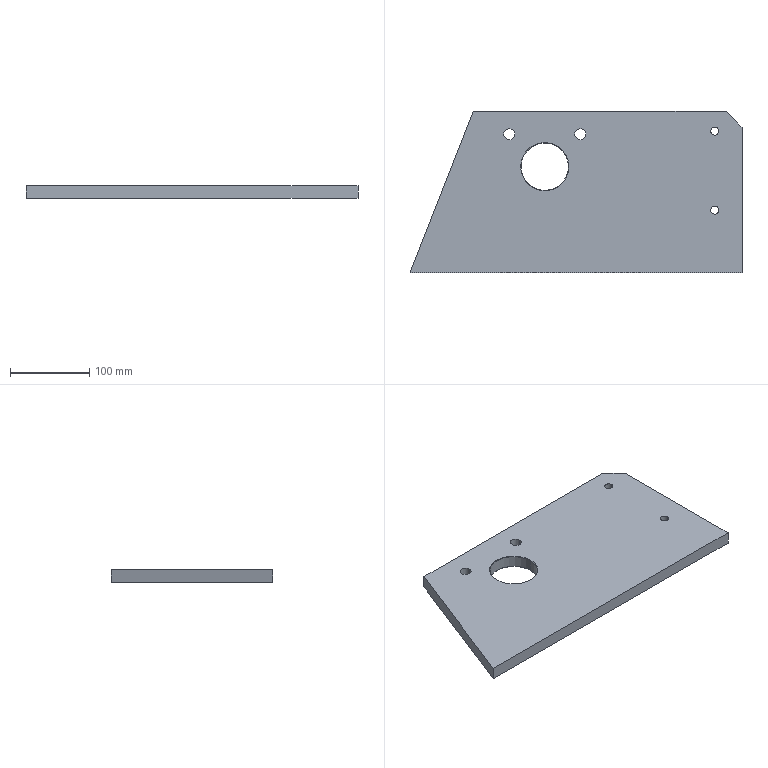Part | STEP file | 03-Vertical plate | 1 solid | 21 faces | box 420 x 204 x 16 mm | volume 1184293 mm3 | cylinder 10 | plane 7 | cone 4 | commonest cylinder face diameters 10.2 x4 14 x4 60 x2